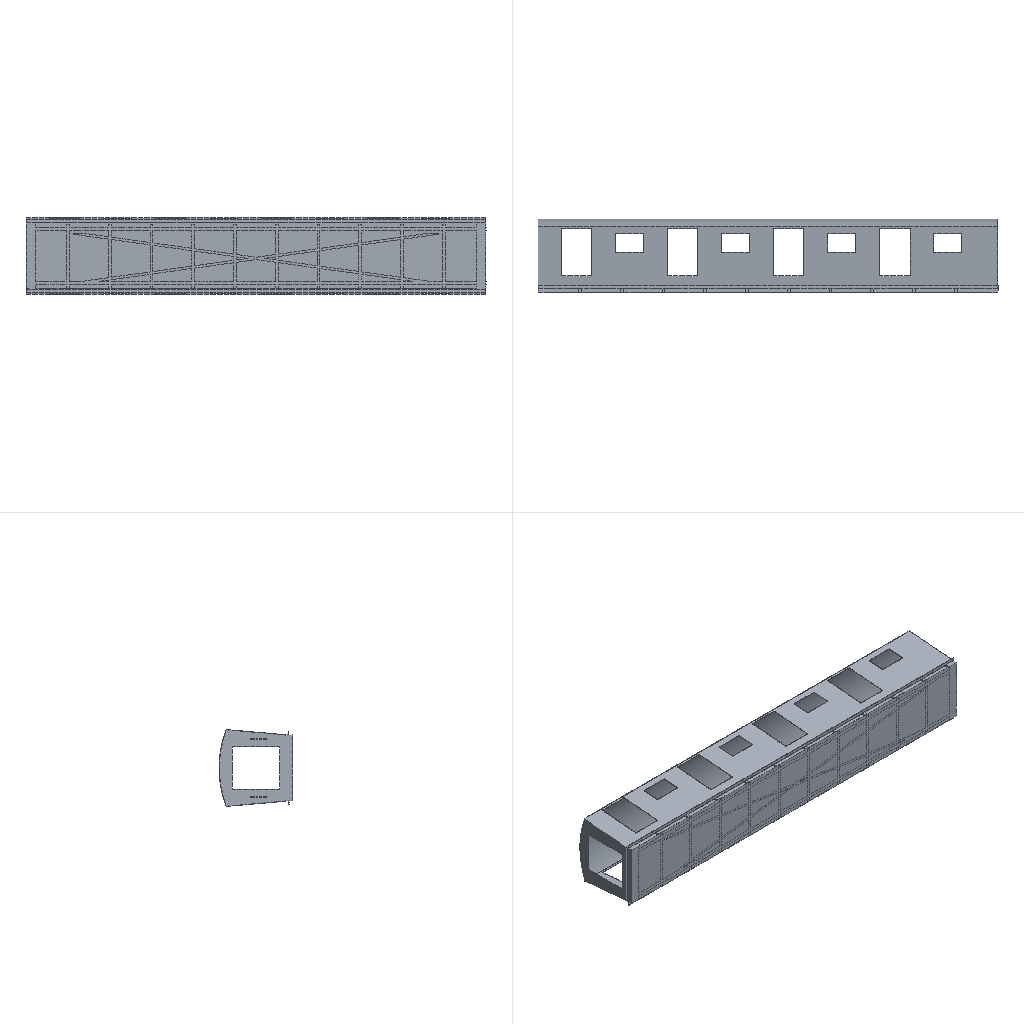Simulation study | ansys workbench
Set-up summary:
category,name,step,type,value,unit,region
solver,ansys_workbench
units,mm-N-s-tonne (MPa),,stated,"/units,MPA"
analysis,LS1,,static
load_step,LS1,LS1,static,nsubst=1; time=1
mesh,nodes,,,381653
mesh,elements,,,228661
element_type,SOLID187,,,187213
element_type,SURF154,,,22856
element_type,TARGE170,,,9296
element_type,CONTA174,,,9296
material,Structural Steel,,E,200000,tonne s^-2 mm^-1
material,Structural Steel,,nu,0.3
material,Structural Steel,,density,7.85e-09,tonne mm^-3
material,Structural Steel,,conductivity,60.5,tonne mm s^-3 C^-1
material,Structural Steel,,specific_heat,4.34e+08,mm^2 s^-2 C^-1
material,Structural Steel,,cte,1.2e-05,C^-1
material,Structural Steel,,permeability,10000
material,Structural Steel,,resistivity,0.00017,ohm mm
load,Define Force Using Surface Effect Elements,LS1,surface-effect pres face 1,0.001087,,SURF154 #13
load,Define Force Using Surface Effect Elements,LS1,surface-effect pres face 2,-0.0007692,,SURF154 #14
bc,Fixed Supports,model,fixed,[dofs=ALL],,_FIXEDSU
contact,Contact Region,,bonded (always),element=CONTA174
contact,Contact Region 2,,bonded (always),element=CONTA174
contact,Contact Region 3,,bonded (always),element=CONTA174
contact,Contact Region 4,,bonded (always),element=CONTA174
named_set,______,,node,2142
named_set,_FIXEDSU,,node,27606
Ansys APDL input file, long lists of numbers shortened:
/batch
/config,noeldb,1     ! force off writing results to database
*get,_wallstrt,active,,time,wall
! ANSYS input file written by Workbench version 2022 R1
! File used for geometry attach:
/title,wbnew--____ (B5)
! ****** Begin Custom Load Command Snippet ******
/COM, ACT Extensions:
/COM,     LSDYNA, 2021.1
/COM,
! ****** End   Custom Load Command Snippet ******
*DIM,_wb_ProjectScratch_dir,string,248
_wb_ProjectScratch_dir(1) = ''
*DIM,_wb_SolverFiles_dir,string,248
_wb_SolverFiles_dir(1) = ''
*DIM,_wb_userfiles_dir,string,248
_wb_userfiles_dir(1) = ''
/com,--- Data in consistent NMM units. See Solving Units in the help system for more information.
/units,MPA
/nopr
/wb,file,start              !  signify a WB generated input file
/prep7
! Turn off shape checking because checks already performed inside WB mesher.
! See help system for more information.
SHPP,OFF,,NOWARN
/nolist
etcon,set             ! allow ANSYS to choose best KEYOP's for 180x elements, resets any applicable keyopt to MAPDL defaults
/com,*********** Nodes for the whole assembly ***********
nblock,3,,419818
(1i9,3e20.9e3)
        1     6.000000000E+00     1.496000000E+03    -1.199650045E+03
! (381652 more lines like these left out)
-1
/wb,elem,start            !  set before creation of elements
/com,*********** Elements for Body 1 "________|NONE" ***********
et,1,187
eblock,19,solid,,148341
(19i9)
        1        1        1        1        0        0        0        0       10        0    38873    84990   125738    85496    90146   169104   172508   169100   169102
! (296681 more lines like these left out)
-1
/com,*********** Elements for Body 2 "___________|NONE" ***********
et,2,187
eblock,19,solid,,5408
(19i9)
        2        2        2        2        0        0        0        0       10        0     5409    13181    13332    13784    13445    20079    21128    20084    20080
! (10815 more lines like these left out)
-1
/com,*********** Elements for Body 3 "___________|NONE[2]" ***********
et,3,187
eblock,19,solid,,5408
(19i9)
        3        3        3        3        0        0        0        0       10        0        1     1130     1281     1733     1394     8028     9077     8033     8029
! (10815 more lines like these left out)
-1
/com,*********** Elements for Body 4 "____3|__-__4[1]" ***********
et,4,187
eblock,19,solid,,28056
(19i9)
        4        4        4        4        0        0        0        0       10        0    10817    25349    25657    33213    33156    42991    45281    42994    42993
! (56111 more lines like these left out)
-1
/wb,elem,end               !  done creating elements
/com,*********** Send User Defined Coordinate System(s) ***********
csys,0
toffst,273.15,  ! Temperature offset from absolute zero
/com,*********** Set Reference Temperature ***********
tref,22.
/wb,mat,start              !  starting to send materials
/com,*********** Send Materials ***********
Temperature = 'TEMP' ! Temperature
MP,DENS,1,7.85e-09,	! tonne mm^-3
MP,ALPX,1,1.2e-05,	! C^-1
MP,C,1,434000000,	! mm^2 s^-2 C^-1
MP,KXX,1,60.5,	! tonne mm s^-3 C^-1
MP,RSVX,1,0.00017,	! ohm mm
MP,EX,1,200000,	! tonne s^-2 mm^-1
MP,NUXY,1,0.3,
MP,MURX,1,10000,
Temperature = 'TEMP' ! Temperature
MP,DENS,2,7.85e-09,	! tonne mm^-3
MP,ALPX,2,1.2e-05,	! C^-1
MP,C,2,434000000,	! mm^2 s^-2 C^-1
MP,KXX,2,60.5,	! tonne mm s^-3 C^-1
MP,RSVX,2,0.00017,	! ohm mm
MP,EX,2,200000,	! tonne s^-2 mm^-1
MP,NUXY,2,0.3,
MP,MURX,2,10000,
Temperature = 'TEMP' ! Temperature
MP,DENS,3,7.85e-09,	! tonne mm^-3
MP,ALPX,3,1.2e-05,	! C^-1
MP,C,3,434000000,	! mm^2 s^-2 C^-1
MP,KXX,3,60.5,	! tonne mm s^-3 C^-1
MP,RSVX,3,0.00017,	! ohm mm
MP,EX,3,200000,	! tonne s^-2 mm^-1
MP,NUXY,3,0.3,
MP,MURX,3,10000,
Temperature = 'TEMP' ! Temperature
MP,DENS,4,7.85e-09,	! tonne mm^-3
MP,ALPX,4,1.2e-05,	! C^-1
MP,C,4,434000000,	! mm^2 s^-2 C^-1
MP,KXX,4,60.5,	! tonne mm s^-3 C^-1
MP,RSVX,4,0.00017,	! ohm mm
MP,EX,4,200000,	! tonne s^-2 mm^-1
MP,NUXY,4,0.3,
MP,MURX,4,10000,
/wb,mat,end                !  done sending materials
!************************* Model Summary ********************
!________|NONE,	结构钢,	matid,	1
!___________|NONE,	结构钢,	matid,	2
!___________|NONE[2],	结构钢,	matid,	3
!____3|__-__4[1],	结构钢,	matid,	4
!************************* End Model Summary ********************
! get the diagonal of the bounding box. Needed later for other things
*get,_xmin,node,,mnloc,x
*get,_ymin,node,,mnloc,y
*get,_zmin,node,,mnloc,z
*get,_xmax,node,,mxloc,x
*get,_ymax,node,,mxloc,y
*get,_zmax,node,,mxloc,z
_ASMDIAG=(_xmax-_xmin)*(_xmax-_xmin)+(_ymax-_ymin)*(_ymax-_ymin)+(_zmax-_zmin)*(_zmax-_zmin)
_ASMDIAG=SQRT(_ASMDIAG)
/wb,contact,start          !  starting to send contact
/com,*********** Create Contact "接触区域" ***********
/com,            Real Constant Set For Above Contact Is 6 & 5
*set,tid,6
*set,cid,5
r,tid
r,cid
et,tid,170
et,cid,174
eblock,10,,,511
(15i9)
   315188        6        6        6        0    91961    92057    93418    93418   204216   204827    93418   204217
! (510 more lines like these left out)
-1
eblock,10,,,511
(15i9)
   315699        5        5        5        0    91961    92057    93418    93418   204216   204827    93418   204217
! (510 more lines like these left out)
-1
eblock,10,,,750
(15i9)
   316210        5        6        5        0    12951    12329    12857    12857    16011    16010    12857    18291
! (749 more lines like these left out)
-1
eblock,10,,,750
(15i9)
   316960        6        5        6        0    12951    12329    12857    12857    16011    16010    12857    18291
! (749 more lines like these left out)
-1
keyo,cid,8,2               ! auto create asymmetric contact (from Program Controlled setting)
keyo,cid,10,0              ! adjust contact stiffness each NR iteration (from Program Controlled setting)
keyo,cid,12,5              ! bonded always
keyo,cid,18,1              ! small sliding turned on by application
keyo,cid,2,0               ! augmented Lagrange (from Program Controlled setting)
keyo,cid,4,0               ! on Gauss point (from Program Controlled setting)
keyo,cid,9,1               ! ignore initial gaps/penetration
keyo,cid,7,0               ! No Prediction
rmod,tid,3,10.      ! FKN
rmod,tid,5,0.       ! ICONT
rmod,tid,6,0.       ! PINB
rmod,tid,10,0.      ! CNOF
rmod,tid,12,0.      ! FKT
rmod,tid,36,35      ! WB DSID
rmod,cid,3,10.      ! FKN
rmod,cid,5,0.       ! ICONT
rmod,cid,6,0.       ! PINB
rmod,cid,10,0.      ! CNOF
rmod,cid,12,0.      ! FKT
rmod,cid,36,35      ! WB DSID
/com,*********** Create Contact "接触区域 2" ***********
/com,            Real Constant Set For Above Contact Is 8 & 7
*set,tid,8
*set,cid,7
r,tid
r,cid
et,tid,170
et,cid,174
eblock,10,,,389
(15i9)
   317710        8        8        8        0    81612    82029    81807    81807   142154   144533    81807   142153
! (388 more lines like these left out)
-1
eblock,10,,,389
(15i9)
   318099        7        7        7        0    81612    82029    81807    81807   142154   144533    81807   142153
! (388 more lines like these left out)
-1
eblock,10,,,1236
(15i9)
   318488        7        8        7        0     1744     1900     2010     2010    11069    11700     2010    11070
! (1235 more lines like these left out)
-1
eblock,10,,,1236
(15i9)
   319724        8        7        8        0     1744     1900     2010     2010    11069    11700     2010    11070
! (1235 more lines like these left out)
-1
keyo,cid,8,2               ! auto create asymmetric contact (from Program Controlled setting)
keyo,cid,10,0              ! adjust contact stiffness each NR iteration (from Program Controlled setting)
keyo,cid,12,5              ! bonded always
keyo,cid,18,1              ! small sliding turned on by application
keyo,cid,2,0               ! augmented Lagrange (from Program Controlled setting)
keyo,cid,4,0               ! on Gauss point (from Program Controlled setting)
keyo,cid,9,1               ! ignore initial gaps/penetration
keyo,cid,7,0               ! No Prediction
rmod,tid,3,10.      ! FKN
rmod,tid,5,0.       ! ICONT
rmod,tid,6,0.       ! PINB
rmod,tid,10,0.      ! CNOF
rmod,tid,12,0.      ! FKT
rmod,tid,36,38      ! WB DSID
rmod,cid,3,10.      ! FKN
rmod,cid,5,0.       ! ICONT
rmod,cid,6,0.       ! PINB
rmod,cid,10,0.      ! CNOF
rmod,cid,12,0.      ! FKT
rmod,cid,36,38      ! WB DSID
/com,*********** Create Contact "接触区域 3" ***********
/com,            Real Constant Set For Above Contact Is 10 & 9
*set,tid,10
*set,cid,9
r,tid
r,cid
et,tid,170
et,cid,174
eblock,10,,,3685
(15i9)
   320960       10       10       10        0   131184   126961   127877   127877   367939   367933   127877   373575
! (3684 more lines like these left out)
-1
eblock,10,,,3685
(15i9)
   324645        9        9        9        0   131184   126961   127877   127877   367939   367933   127877   373575
! (3684 more lines like these left out)
-1
eblock,10,,,2519
(15i9)
   328330        9       10        9        0    24186    29340    29257    29257    34181    64024    29257    34180
! (2518 more lines like these left out)
-1
eblock,10,,,2519
(15i9)
   330849       10        9       10        0    24186    29340    29257    29257    34181    64024    29257    34180
! (2518 more lines like these left out)
-1
keyo,cid,8,2               ! auto create asymmetric contact (from Program Controlled setting)
keyo,cid,10,0              ! adjust contact stiffness each NR iteration (from Program Controlled setting)
keyo,cid,12,5              ! bonded always
keyo,cid,18,1              ! small sliding turned on by application
keyo,cid,2,0               ! augmented Lagrange (from Program Controlled setting)
keyo,cid,4,0               ! on Gauss point (from Program Controlled setting)
keyo,cid,9,1               ! ignore initial gaps/penetration
keyo,cid,7,0               ! No Prediction
rmod,tid,3,10.      ! FKN
rmod,tid,5,0.       ! ICONT
rmod,tid,6,0.       ! PINB
rmod,tid,10,0.      ! CNOF
rmod,tid,12,0.      ! FKT
rmod,tid,36,41      ! WB DSID
rmod,cid,3,10.      ! FKN
rmod,cid,5,0.       ! ICONT
rmod,cid,6,0.       ! PINB
rmod,cid,10,0.      ! CNOF
rmod,cid,12,0.      ! FKT
rmod,cid,36,41      ! WB DSID
/com,*********** Create Contact "接触区域 4" ***********
/com,            Real Constant Set For Above Contact Is 12 & 11
*set,tid,12
*set,cid,11
r,tid
r,cid
et,tid,170
et,cid,174
eblock,10,,,116
(15i9)
   333368       12       12       12        0    12938    12319    12407    12407    15946    15943    12407    16511
! (115 more lines like these left out)
-1
eblock,10,,,116
(15i9)
   333484       11       11       11        0    12938    12319    12407    12407    15946    15943    12407    16511
! (115 more lines like these left out)
-1
eblock,10,,,90
(15i9)
   333600       11       12       11        0    28522    29325    28528    28528    61006    61039    28528    61004
! (89 more lines like these left out)
-1
eblock,10,,,90
(15i9)
   333690       12       11       12        0    28522    29325    28528    28528    61006    61039    28528    61004
! (89 more lines like these left out)
-1
keyo,cid,8,2               ! auto create asymmetric contact (from Program Controlled setting)
keyo,cid,10,0              ! adjust contact stiffness each NR iteration (from Program Controlled setting)
keyo,cid,12,5              ! bonded always
keyo,cid,18,1              ! small sliding turned on by application
keyo,cid,2,0               ! augmented Lagrange (from Program Controlled setting)
keyo,cid,4,0               ! on Gauss point (from Program Controlled setting)
keyo,cid,9,1               ! ignore initial gaps/penetration
keyo,cid,7,0               ! No Prediction
rmod,tid,3,10.      ! FKN
rmod,tid,5,0.       ! ICONT
rmod,tid,6,0.       ! PINB
rmod,tid,10,0.      ! CNOF
rmod,tid,12,0.      ! FKT
rmod,tid,36,44      ! WB DSID
rmod,cid,3,10.      ! FKN
rmod,cid,5,0.       ! ICONT
rmod,cid,6,0.       ! PINB
rmod,cid,10,0.      ! CNOF
rmod,cid,12,0.      ! FKT
rmod,cid,36,44      ! WB DSID
nsel,all
esel,all
/wb,contact,end            !  done creating contacts
/com,*********** Send Named Selection as Node Component ***********
CMBLOCK,______  ,NODE,     2142
(8i10)
       217       218       219       220       221       222       223       224
! (267 more lines like these left out)
/golist
/wb,load,start             !  starting to send loads
/com,*********** Fixed Supports ***********
CMBLOCK,_FIXEDSU,NODE,    27606
(8i10)
       217       218       219       220       221       222       223       224
! (3450 more lines like these left out)
cmsel,s,_FIXEDSU
d,all,all
nsel,all
/com,*********** Define Force Using Surface Effect Elements ***********
local,12,0,0.,0.,0.,0.,0.,0.
csys,0
et,13,154
eblock,10,,,1460
(15i9)
   333780       13       13       13       12     1744     1900     2010     2010    11069    11700     2010    11070
! (1459 more lines like these left out)
-1
esel,s,type,,13
keyop,13,2,1                ! Apply load in local coordinate system
keyop,13,7,1                ! Use original area so load is constant in large deformation
esel,all
/com,*********** Define Force Using Surface Effect Elements ***********
local,13,0,0.,0.,0.,0.,0.,0.
csys,0
et,14,154
eblock,10,,,21396
(15i9)
   335240       14       14       14       13    83460   105268   104947   104947   159183   258638   104947   159181
! (21395 more lines like these left out)
-1
esel,s,type,,14
keyop,14,2,1                ! Apply load in local coordinate system
keyop,14,7,1                ! Use original area so load is constant in large deformation
esel,all
/gst,on,on
fini
*get,_numnode,node,0,count
*get,_numelem,elem,0,count
*get, _MAXELEMNUM, elem, 0, NUM, MAX
*get, _MAXNODENUM, node, 0, NUM, MAX
*get, _MAXELEMTYPE, etyp, 0, NUM, MAX
*get, _MAXREALCONST, real, 0, NUM, MAX
/go
/wb,load,end               !  done creating loads
/com,--- Number of total nodes = %_numnode%
/com,--- Number of contact elements = 41448
/com,--- Number of spring elements = 0
/com,--- Number of bearing elements = 0
/com,--- Number of solid elements = 187213
/com,--- Number of condensed parts = 0
/com,--- Number of total elements = %_numelem%
*get,_wallbsol,active,,time,wall
/com,****************************************************************************
/com,*************************    SOLUTION       ********************************
/com,****************************************************************************
/solu
antype,0                   ! static analysis
_thickRatio=  0     ! Ratio of thick parts in the model
eqsl,sparse,,,,,1
cntr,print,1               ! print out contact info and also make no initial contact an error
dmpoption,emat,no             ! Don't combine emat file for DANSYS
dmpoption,esav,no             ! Don't combine esav file for DANSYS
nldiag,cont,iter           ! print out contact info each equilibrium iteration
rescontrol,,none                 ! Do not keep any restart files
/com,****************************************************
/com,******************* SOLVE FOR LS 1 OF 1 ****************
esel,s,type,,13
nsle
sfe,all,1,pres,1,1.0872592559787e-003
sfe,all,2,pres,1,0.
sfe,all,3,pres,1,0.
esel,s,type,,14
nsle
sfe,all,1,pres,1,0.
sfe,all,2,pres,1,-7.69197156633482e-004
sfe,all,3,pres,1,0.
nsel,all
esel,all
/nopr
/gopr
nsub,1,1,1
time,1.
outres,erase
outres,all,none
outres,nsol,all,
outres,rsol,all
outres,eangl,all
outres,etmp,all
outres,veng,all
outres,strs,all,
outres,epel,all,
outres,eppl,all,
outres,cont,all,
! *********** WB SOLVE COMMAND ***********
! check interactive state
*get,ANSINTER_,active,,int
*if,ANSINTER_,ne,0,then
/eof
*endif
solve
/com *************** Write FE CONNECTORS *********
CEWRITE,file,ce,,INTE
/com,****************************************************
/com,*************** FINISHED SOLVE FOR LS 1 *************
*get,_wallasol,active,,time,wall
/nopr
*get,_numnode,node,0,count
*get,_numelem,elem,0,count
*get, _MAXELEMNUM, elem, 0, NUM, MAX
*get, _MAXNODENUM, node, 0, NUM, MAX,,,INTERNAL
*get, _MAXELEMTYPE, etyp, 0, NUM, MAX
*get, _MAXREALCONST, real, 0, NUM, MAX
/gopr
/post1
xmlo,ENCODING,ISO-8859-1
xmlo,parm
/xml,parm,xml
fini
/gopr
*get,_walldone,active,,time,wall
_preptime=(_wallbsol-_wallstrt)*3600
_solvtime=(_wallasol-_wallbsol)*3600
_posttime=(_walldone-_wallasol)*3600
_totaltim=(_walldone-_wallstrt)*3600
*get,_dlbratio,active,0,solu,dlbr
*get,_combtime,active,0,solu,comb
*get,_ssmode,active,0,solu,ssmm
*get,_ndofs,active,0,solu,ndof
*get,_sol_end_time,active,0,set,time
*if,_sol_end_time,eq,1.,then
/fclean				!clean distributed files
*endif
/com,--- Total number of nodes = %_numnode%
/com,--- Total number of elements = %_numelem%
/com,--- Element load balance ratio = %_dlbratio%
/com,--- Time to combine distributed files = %_combtime%
/com,--- Sparse memory mode = %_ssmode%
/com,--- Number of DOF = %_ndofs%
/wb,file,end               ! done with WB generated input
Results summary:
result,analyses[0].index,,,1
result,analyses[0].system,,,SYS
result,analyses[0].deck,,,deck.dat
result,analyses[0].solve_status,,,completed
result,analyses[0].analysis_type,,,static
result,analyses[0].physics,,,mechanical
result,analyses[0].unit_system,,,"NMM: mm, ton, N, s, mV, mA, degC"
result,analyses[0].n_sets,,,1
result,analyses[0].load_steps[0].set,set=1,,1
result,analyses[0].load_steps[0].time_or_freq,set=1,,1
result,analyses[0].load_steps[0].max_displacement_magnitude,set=1,,30.256
result,analyses[0].load_steps[0].max_von_mises_nodal,set=1,,71.832
result,analyses[0].load_steps[0].reaction_force_sum_xyz[1],set=1,,-5000
result,analyses[0].load_steps[0].reaction_force_sum_xyz[2],set=1,,49999.7
result,analyses[0].load_steps[0].reaction_force_sum_xyz[3],set=1,,0.001647